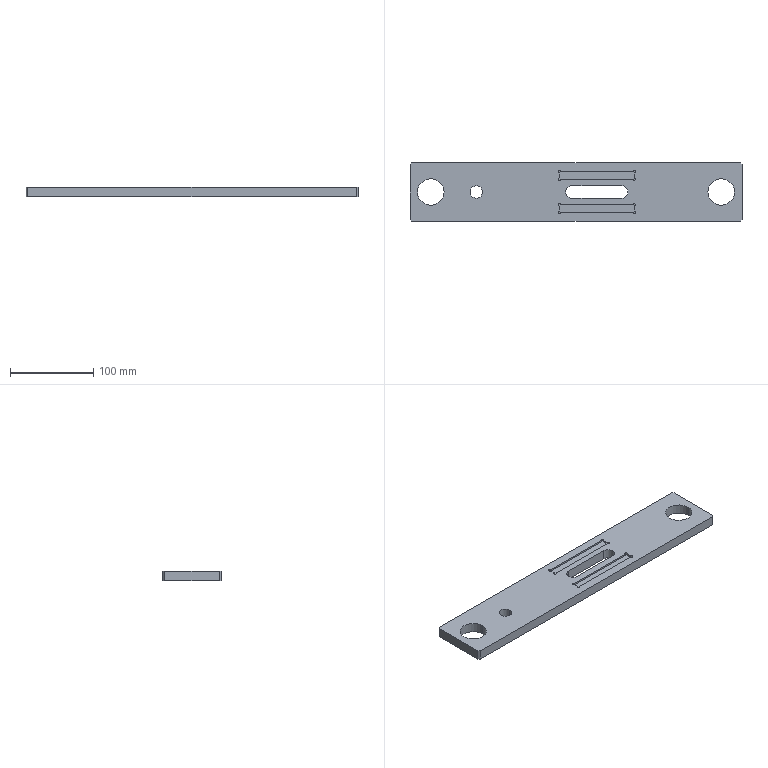Part | STEP file | 001-006-Pre-insertion mechanism pressure plate | 1 solid | 43 faces | box 400 x 70 x 12 mm | volume 298236 mm3 | plane 22 | cylinder 21 | commonest cylinder face diameters 3 x12 15 x5 32 x4